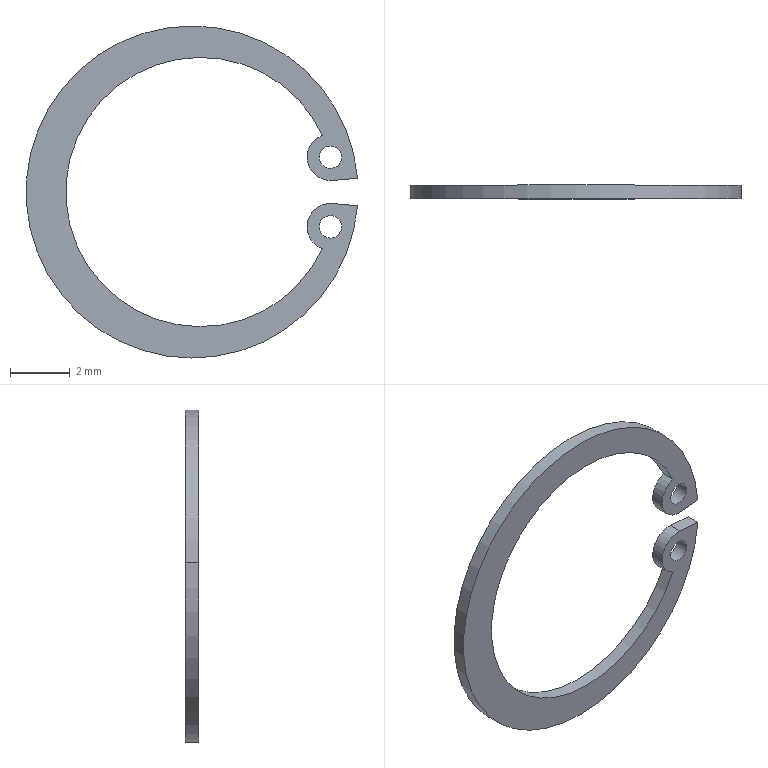Part | STEP file | 2026.6.15-Main Assembly图.sldasm-Part-286 | 1 solid | 16 faces | box 11.081 x 0.45 x 11.1 mm | volume 15.053 mm3 | cylinder 12 | plane 4 | commonest cylinder face diameters 0.75 x4 1.56 x4 9 x2 11.1 x2
STEP:
#1=CARTESIAN_POINT('',(-1507.657,1426.544,3408.546));
#2=VERTEX_POINT('',#1);
#3=CARTESIAN_POINT('',(-1508.494,1426.544,3408.473));
#4=VERTEX_POINT('',#3);
#5=CARTESIAN_POINT('',(-1508.494,1426.544,3408.473));
#6=DIRECTION('',(-0.9962,0.,-0.08716));
#7=VECTOR('',#6,1000.);
#8=LINE('',#5,#7);
#9=EDGE_CURVE('',#2,#4,#8,.T.);
#10=ORIENTED_EDGE('',*,*,#9,.T.);
#11=CARTESIAN_POINT('',(-1509.34,1426.544,3409.311));
#12=VERTEX_POINT('',#11);
#13=CARTESIAN_POINT('',(-1508.562,1426.544,3409.25));
#14=DIRECTION('',(0.,-1.,0.));
#15=DIRECTION('',(-0.9969,0.,0.0785));
#16=AXIS2_PLACEMENT_3D('',#13,#14,#15);
#17=CIRCLE('',#16,0.78);
#18=EDGE_CURVE('',#12,#4,#17,.T.);
#19=ORIENTED_EDGE('',*,*,#18,.F.);
#20=CARTESIAN_POINT('',(-1508.828,1426.544,3409.983));
#21=VERTEX_POINT('',#20);
#22=CARTESIAN_POINT('',(-1508.562,1426.544,3409.25));
#23=DIRECTION('',(0.,-1.,0.));
#24=DIRECTION('',(-0.9969,0.,0.0785));
#25=AXIS2_PLACEMENT_3D('',#22,#23,#24);
#26=CIRCLE('',#25,0.78);
#27=EDGE_CURVE('',#21,#12,#26,.T.);
#28=ORIENTED_EDGE('',*,*,#27,.F.);
#29=CARTESIAN_POINT('',(-1517.395,1426.544,3408.44));
#30=VERTEX_POINT('',#29);
#31=CARTESIAN_POINT('',(-1512.909,1426.544,3408.086));
#32=DIRECTION('',(0.,-1.,0.));
#33=DIRECTION('',(-0.9969,0.,0.0785));
#34=AXIS2_PLACEMENT_3D('',#31,#32,#33);
#35=CIRCLE('',#34,4.5);
#36=EDGE_CURVE('',#21,#30,#35,.T.);
#37=ORIENTED_EDGE('',*,*,#36,.T.);
#38=CARTESIAN_POINT('',(-1508.828,1426.544,3406.19));
#39=VERTEX_POINT('',#38);
#40=CARTESIAN_POINT('',(-1512.909,1426.544,3408.086));
#41=DIRECTION('',(0.,-1.,0.));
#42=DIRECTION('',(-0.9969,0.,0.0785));
#43=AXIS2_PLACEMENT_3D('',#40,#41,#42);
#44=CIRCLE('',#43,4.5);
#45=EDGE_CURVE('',#30,#39,#44,.T.);
#46=ORIENTED_EDGE('',*,*,#45,.T.);
#47=CARTESIAN_POINT('',(-1509.34,1426.544,3406.984));
#48=VERTEX_POINT('',#47);
#49=CARTESIAN_POINT('',(-1508.562,1426.544,3406.923));
#50=DIRECTION('',(0.,-1.,0.));
#51=DIRECTION('',(-0.9969,0.,0.0785));
#52=AXIS2_PLACEMENT_3D('',#49,#50,#51);
#53=CIRCLE('',#52,0.78);
#54=EDGE_CURVE('',#48,#39,#53,.T.);
#55=ORIENTED_EDGE('',*,*,#54,.F.);
#56=CARTESIAN_POINT('',(-1508.494,1426.544,3407.7));
#57=VERTEX_POINT('',#56);
#58=CARTESIAN_POINT('',(-1508.562,1426.544,3406.923));
#59=DIRECTION('',(0.,-1.,0.));
#60=DIRECTION('',(-0.9969,0.,0.0785));
#61=AXIS2_PLACEMENT_3D('',#58,#59,#60);
#62=CIRCLE('',#61,0.78);
#63=EDGE_CURVE('',#57,#48,#62,.T.);
#64=ORIENTED_EDGE('',*,*,#63,.F.);
#65=CARTESIAN_POINT('',(-1507.657,1426.544,3407.627));
#66=VERTEX_POINT('',#65);
#67=CARTESIAN_POINT('',(-1508.494,1426.544,3407.7));
#68=DIRECTION('',(0.9962,0.,-0.08716));
#69=VECTOR('',#68,1000.);
#70=LINE('',#67,#69);
#71=EDGE_CURVE('',#57,#66,#70,.T.);
#72=ORIENTED_EDGE('',*,*,#71,.T.);
#73=CARTESIAN_POINT('',(-1518.721,1426.544,3408.522));
#74=VERTEX_POINT('',#73);
#75=CARTESIAN_POINT('',(-1513.188,1426.544,3408.086));
#76=DIRECTION('',(0.,-1.,0.));
#77=DIRECTION('',(-0.9969,0.,0.0785));
#78=AXIS2_PLACEMENT_3D('',#75,#76,#77);
#79=CIRCLE('',#78,5.55);
#80=EDGE_CURVE('',#74,#66,#79,.T.);
#81=ORIENTED_EDGE('',*,*,#80,.F.);
#82=CARTESIAN_POINT('',(-1513.188,1426.544,3408.086));
#83=DIRECTION('',(0.,-1.,0.));
#84=DIRECTION('',(-0.9969,0.,0.0785));
#85=AXIS2_PLACEMENT_3D('',#82,#83,#84);
#86=CIRCLE('',#85,5.55);
#87=EDGE_CURVE('',#2,#74,#86,.T.);
#88=ORIENTED_EDGE('',*,*,#87,.F.);
#89=EDGE_LOOP('',(#10,#19,#28,#37,#46,#55,#64,#72,#81,#88));
#90=FACE_OUTER_BOUND('',#89,.T.);
#91=CARTESIAN_POINT('',(-1508.936,1426.544,3406.952));
#92=VERTEX_POINT('',#91);
#93=CARTESIAN_POINT('',(-1508.188,1426.544,3406.894));
#94=VERTEX_POINT('',#93);
#95=CARTESIAN_POINT('',(-1508.562,1426.544,3406.923));
#96=DIRECTION('',(0.,-1.,0.));
#97=DIRECTION('',(-0.9969,0.,0.0785));
#98=AXIS2_PLACEMENT_3D('',#95,#96,#97);
#99=CIRCLE('',#98,0.375);
#100=EDGE_CURVE('',#92,#94,#99,.T.);
#101=ORIENTED_EDGE('',*,*,#100,.T.);
#102=CARTESIAN_POINT('',(-1508.562,1426.544,3406.923));
#103=DIRECTION('',(0.,-1.,0.));
#104=DIRECTION('',(-0.9969,0.,0.0785));
#105=AXIS2_PLACEMENT_3D('',#102,#103,#104);
#106=CIRCLE('',#105,0.375);
#107=EDGE_CURVE('',#94,#92,#106,.T.);
#108=ORIENTED_EDGE('',*,*,#107,.T.);
#109=EDGE_LOOP('',(#101,#108));
#110=FACE_BOUND('',#109,.T.);
#111=CARTESIAN_POINT('',(-1508.936,1426.544,3409.279));
#112=VERTEX_POINT('',#111);
#113=CARTESIAN_POINT('',(-1508.188,1426.544,3409.22));
#114=VERTEX_POINT('',#113);
#115=CARTESIAN_POINT('',(-1508.562,1426.544,3409.25));
#116=DIRECTION('',(0.,-1.,0.));
#117=DIRECTION('',(-0.9969,0.,0.0785));
#118=AXIS2_PLACEMENT_3D('',#115,#116,#117);
#119=CIRCLE('',#118,0.375);
#120=EDGE_CURVE('',#112,#114,#119,.T.);
#121=ORIENTED_EDGE('',*,*,#120,.T.);
#122=CARTESIAN_POINT('',(-1508.562,1426.544,3409.25));
#123=DIRECTION('',(0.,-1.,0.));
#124=DIRECTION('',(-0.9969,0.,0.0785));
#125=AXIS2_PLACEMENT_3D('',#122,#123,#124);
#126=CIRCLE('',#125,0.375);
#127=EDGE_CURVE('',#114,#112,#126,.T.);
#128=ORIENTED_EDGE('',*,*,#127,.T.);
#129=EDGE_LOOP('',(#121,#128));
#130=FACE_BOUND('',#129,.T.);
#131=CARTESIAN_POINT('',(-1513.188,1426.544,3408.086));
#132=DIRECTION('',(0.,1.,0.));
#133=DIRECTION('',(0.,0.,-1.));
#134=AXIS2_PLACEMENT_3D('',#131,#132,#133);
#135=PLANE('',#134);
#136=ADVANCED_FACE('',(#90,#110,#130),#135,.T.);
#137=CARTESIAN_POINT('',(-1518.721,1426.094,3408.522));
#138=VERTEX_POINT('',#137);
#139=CARTESIAN_POINT('',(-1518.721,1426.094,3408.522));
#140=DIRECTION('',(0.,-1.,0.));
#141=VECTOR('',#140,1000.);
#142=LINE('',#139,#141);
#143=EDGE_CURVE('',#74,#138,#142,.T.);
#144=ORIENTED_EDGE('',*,*,#143,.F.);
#145=ORIENTED_EDGE('',*,*,#80,.T.);
#146=CARTESIAN_POINT('',(-1507.657,1426.094,3407.627));
#147=VERTEX_POINT('',#146);
#148=CARTESIAN_POINT('',(-1507.657,1406.528,3407.627));
#149=DIRECTION('',(0.,-1.,0.));
#150=VECTOR('',#149,1000.);
#151=LINE('',#148,#150);
#152=EDGE_CURVE('',#66,#147,#151,.T.);
#153=ORIENTED_EDGE('',*,*,#152,.T.);
#154=CARTESIAN_POINT('',(-1513.188,1426.094,3408.086));
#155=DIRECTION('',(0.,1.,0.));
#156=DIRECTION('',(-0.9969,0.,0.0785));
#157=AXIS2_PLACEMENT_3D('',#154,#155,#156);
#158=CIRCLE('',#157,5.55);
#159=EDGE_CURVE('',#147,#138,#158,.T.);
#160=ORIENTED_EDGE('',*,*,#159,.T.);
#161=EDGE_LOOP('',(#144,#145,#153,#160));
#162=FACE_OUTER_BOUND('',#161,.T.);
#163=CARTESIAN_POINT('',(-1513.188,1426.094,3408.086));
#164=DIRECTION('',(0.,-1.,0.));
#165=DIRECTION('',(0.9969,0.,-0.0785));
#166=AXIS2_PLACEMENT_3D('',#163,#164,#165);
#167=CYLINDRICAL_SURFACE('',#166,5.55);
#168=ADVANCED_FACE('',(#162),#167,.T.);
#169=CARTESIAN_POINT('',(-1508.494,1426.094,3408.473));
#170=VERTEX_POINT('',#169);
#171=CARTESIAN_POINT('',(-1508.494,1406.528,3408.473));
#172=DIRECTION('',(0.,-1.,0.));
#173=VECTOR('',#172,1000.);
#174=LINE('',#171,#173);
#175=EDGE_CURVE('',#4,#170,#174,.T.);
#176=ORIENTED_EDGE('',*,*,#175,.F.);
#177=ORIENTED_EDGE('',*,*,#9,.F.);
#178=CARTESIAN_POINT('',(-1507.657,1426.094,3408.546));
#179=VERTEX_POINT('',#178);
#180=CARTESIAN_POINT('',(-1507.657,1406.528,3408.546));
#181=DIRECTION('',(0.,1.,0.));
#182=VECTOR('',#181,1000.);
#183=LINE('',#180,#182);
#184=EDGE_CURVE('',#179,#2,#183,.T.);
#185=ORIENTED_EDGE('',*,*,#184,.F.);
#186=CARTESIAN_POINT('',(-1507.657,1426.094,3408.546));
#187=DIRECTION('',(-0.9962,0.,-0.08716));
#188=VECTOR('',#187,1000.);
#189=LINE('',#186,#188);
#190=EDGE_CURVE('',#179,#170,#189,.T.);
#191=ORIENTED_EDGE('',*,*,#190,.T.);
#192=EDGE_LOOP('',(#176,#177,#185,#191));
#193=FACE_OUTER_BOUND('',#192,.T.);
#194=CARTESIAN_POINT('',(-1508.494,1406.528,3408.473));
#195=DIRECTION('',(-0.08716,0.,0.9962));
#196=DIRECTION('',(0.,1.,0.));
#197=AXIS2_PLACEMENT_3D('',#194,#195,#196);
#198=PLANE('',#197);
#199=ADVANCED_FACE('',(#193),#198,.F.);
#200=CARTESIAN_POINT('',(-1509.34,1426.094,3409.311));
#201=VERTEX_POINT('',#200);
#202=CARTESIAN_POINT('',(-1509.34,1406.528,3409.311));
#203=DIRECTION('',(0.,-1.,0.));
#204=VECTOR('',#203,1000.);
#205=LINE('',#202,#204);
#206=EDGE_CURVE('',#12,#201,#205,.T.);
#207=ORIENTED_EDGE('',*,*,#206,.F.);
#208=ORIENTED_EDGE('',*,*,#18,.T.);
#209=ORIENTED_EDGE('',*,*,#175,.T.);
#210=CARTESIAN_POINT('',(-1508.562,1426.094,3409.25));
#211=DIRECTION('',(0.,1.,0.));
#212=DIRECTION('',(-0.9969,0.,0.0785));
#213=AXIS2_PLACEMENT_3D('',#210,#211,#212);
#214=CIRCLE('',#213,0.78);
#215=EDGE_CURVE('',#170,#201,#214,.T.);
#216=ORIENTED_EDGE('',*,*,#215,.T.);
#217=EDGE_LOOP('',(#207,#208,#209,#216));
#218=FACE_OUTER_BOUND('',#217,.T.);
#219=CARTESIAN_POINT('',(-1508.562,1406.528,3409.25));
#220=DIRECTION('',(0.,-1.,0.));
#221=DIRECTION('',(0.9969,0.,-0.0785));
#222=AXIS2_PLACEMENT_3D('',#219,#220,#221);
#223=CYLINDRICAL_SURFACE('',#222,0.78);
#224=ADVANCED_FACE('',(#218),#223,.T.);
#225=CARTESIAN_POINT('',(-1517.395,1426.094,3408.44));
#226=VERTEX_POINT('',#225);
#227=CARTESIAN_POINT('',(-1517.395,1406.528,3408.44));
#228=DIRECTION('',(0.,-1.,0.));
#229=VECTOR('',#228,1000.);
#230=LINE('',#227,#229);
#231=EDGE_CURVE('',#30,#226,#230,.T.);
#232=ORIENTED_EDGE('',*,*,#231,.F.);
#233=ORIENTED_EDGE('',*,*,#36,.F.);
#234=CARTESIAN_POINT('',(-1508.828,1426.094,3409.983));
#235=VERTEX_POINT('',#234);
#236=CARTESIAN_POINT('',(-1508.828,1406.528,3409.983));
#237=DIRECTION('',(0.,1.,0.));
#238=VECTOR('',#237,1000.);
#239=LINE('',#236,#238);
#240=EDGE_CURVE('',#235,#21,#239,.T.);
#241=ORIENTED_EDGE('',*,*,#240,.F.);
#242=CARTESIAN_POINT('',(-1512.909,1426.094,3408.086));
#243=DIRECTION('',(0.,-1.,0.));
#244=DIRECTION('',(-0.9969,0.,0.0785));
#245=AXIS2_PLACEMENT_3D('',#242,#243,#244);
#246=CIRCLE('',#245,4.5);
#247=EDGE_CURVE('',#235,#226,#246,.T.);
#248=ORIENTED_EDGE('',*,*,#247,.T.);
#249=EDGE_LOOP('',(#232,#233,#241,#248));
#250=FACE_OUTER_BOUND('',#249,.T.);
#251=CARTESIAN_POINT('',(-1512.909,1406.528,3408.086));
#252=DIRECTION('',(0.,-1.,0.));
#253=DIRECTION('',(0.9969,0.,-0.0785));
#254=AXIS2_PLACEMENT_3D('',#251,#252,#253);
#255=CYLINDRICAL_SURFACE('',#254,4.5);
#256=ADVANCED_FACE('',(#250),#255,.F.);
#257=CARTESIAN_POINT('',(-1509.34,1426.094,3406.984));
#258=VERTEX_POINT('',#257);
#259=CARTESIAN_POINT('',(-1509.34,1406.528,3406.984));
#260=DIRECTION('',(0.,-1.,0.));
#261=VECTOR('',#260,1000.);
#262=LINE('',#259,#261);
#263=EDGE_CURVE('',#48,#258,#262,.T.);
#264=ORIENTED_EDGE('',*,*,#263,.F.);
#265=ORIENTED_EDGE('',*,*,#54,.T.);
#266=CARTESIAN_POINT('',(-1508.828,1426.094,3406.19));
#267=VERTEX_POINT('',#266);
#268=CARTESIAN_POINT('',(-1508.828,1406.528,3406.19));
#269=DIRECTION('',(0.,-1.,0.));
#270=VECTOR('',#269,1000.);
#271=LINE('',#268,#270);
#272=EDGE_CURVE('',#39,#267,#271,.T.);
#273=ORIENTED_EDGE('',*,*,#272,.T.);
#274=CARTESIAN_POINT('',(-1508.562,1426.094,3406.923));
#275=DIRECTION('',(0.,1.,0.));
#276=DIRECTION('',(-0.9969,0.,0.0785));
#277=AXIS2_PLACEMENT_3D('',#274,#275,#276);
#278=CIRCLE('',#277,0.78);
#279=EDGE_CURVE('',#267,#258,#278,.T.);
#280=ORIENTED_EDGE('',*,*,#279,.T.);
#281=EDGE_LOOP('',(#264,#265,#273,#280));
#282=FACE_OUTER_BOUND('',#281,.T.);
#283=CARTESIAN_POINT('',(-1508.562,1406.528,3406.923));
#284=DIRECTION('',(0.,-1.,0.));
#285=DIRECTION('',(0.9969,0.,-0.0785));
#286=AXIS2_PLACEMENT_3D('',#283,#284,#285);
#287=CYLINDRICAL_SURFACE('',#286,0.78);
#288=ADVANCED_FACE('',(#282),#287,.T.);
#289=CARTESIAN_POINT('',(-1508.494,1426.094,3407.7));
#290=VERTEX_POINT('',#289);
#291=CARTESIAN_POINT('',(-1508.494,1406.528,3407.7));
#292=DIRECTION('',(0.,1.,0.));
#293=VECTOR('',#292,1000.);
#294=LINE('',#291,#293);
#295=EDGE_CURVE('',#290,#57,#294,.T.);
#296=ORIENTED_EDGE('',*,*,#295,.F.);
#297=CARTESIAN_POINT('',(-1508.494,1426.094,3407.7));
#298=DIRECTION('',(0.9962,0.,-0.08716));
#299=VECTOR('',#298,1000.);
#300=LINE('',#297,#299);
#301=EDGE_CURVE('',#290,#147,#300,.T.);
#302=ORIENTED_EDGE('',*,*,#301,.T.);
#303=ORIENTED_EDGE('',*,*,#152,.F.);
#304=ORIENTED_EDGE('',*,*,#71,.F.);
#305=EDGE_LOOP('',(#296,#302,#303,#304));
#306=FACE_OUTER_BOUND('',#305,.T.);
#307=CARTESIAN_POINT('',(-1508.494,1406.528,3407.7));
#308=DIRECTION('',(-0.08716,0.,-0.9962));
#309=DIRECTION('',(0.,1.,0.));
#310=AXIS2_PLACEMENT_3D('',#307,#308,#309);
#311=PLANE('',#310);
#312=ADVANCED_FACE('',(#306),#311,.F.);
#313=CARTESIAN_POINT('',(-1508.188,1426.094,3406.894));
#314=VERTEX_POINT('',#313);
#315=CARTESIAN_POINT('',(-1508.188,1410.854,3406.894));
#316=DIRECTION('',(0.,1.,0.));
#317=VECTOR('',#316,1000.);
#318=LINE('',#315,#317);
#319=EDGE_CURVE('',#314,#94,#318,.T.);
#320=ORIENTED_EDGE('',*,*,#319,.T.);
#321=ORIENTED_EDGE('',*,*,#100,.F.);
#322=CARTESIAN_POINT('',(-1508.936,1426.094,3406.952));
#323=VERTEX_POINT('',#322);
#324=CARTESIAN_POINT('',(-1508.936,1410.854,3406.952));
#325=DIRECTION('',(0.,1.,0.));
#326=VECTOR('',#325,1000.);
#327=LINE('',#324,#326);
#328=EDGE_CURVE('',#323,#92,#327,.T.);
#329=ORIENTED_EDGE('',*,*,#328,.F.);
#330=CARTESIAN_POINT('',(-1508.562,1426.094,3406.923));
#331=DIRECTION('',(0.,-1.,0.));
#332=DIRECTION('',(-0.9969,0.,0.0785));
#333=AXIS2_PLACEMENT_3D('',#330,#331,#332);
#334=CIRCLE('',#333,0.375);
#335=EDGE_CURVE('',#323,#314,#334,.T.);
#336=ORIENTED_EDGE('',*,*,#335,.T.);
#337=EDGE_LOOP('',(#320,#321,#329,#336));
#338=FACE_OUTER_BOUND('',#337,.T.);
#339=CARTESIAN_POINT('',(-1508.562,1410.854,3406.923));
#340=DIRECTION('',(0.,-1.,0.));
#341=DIRECTION('',(0.9969,0.,-0.0785));
#342=AXIS2_PLACEMENT_3D('',#339,#340,#341);
#343=CYLINDRICAL_SURFACE('',#342,0.375);
#344=ADVANCED_FACE('',(#338),#343,.F.);
#345=CARTESIAN_POINT('',(-1508.188,1426.094,3409.22));
#346=VERTEX_POINT('',#345);
#347=CARTESIAN_POINT('',(-1508.188,1410.854,3409.22));
#348=DIRECTION('',(0.,1.,0.));
#349=VECTOR('',#348,1000.);
#350=LINE('',#347,#349);
#351=EDGE_CURVE('',#346,#114,#350,.T.);
#352=ORIENTED_EDGE('',*,*,#351,.T.);
#353=ORIENTED_EDGE('',*,*,#120,.F.);
#354=CARTESIAN_POINT('',(-1508.936,1426.094,3409.279));
#355=VERTEX_POINT('',#354);
#356=CARTESIAN_POINT('',(-1508.936,1410.854,3409.279));
#357=DIRECTION('',(0.,1.,0.));
#358=VECTOR('',#357,1000.);
#359=LINE('',#356,#358);
#360=EDGE_CURVE('',#355,#112,#359,.T.);
#361=ORIENTED_EDGE('',*,*,#360,.F.);
#362=CARTESIAN_POINT('',(-1508.562,1426.094,3409.25));
#363=DIRECTION('',(0.,-1.,0.));
#364=DIRECTION('',(-0.9969,0.,0.0785));
#365=AXIS2_PLACEMENT_3D('',#362,#363,#364);
#366=CIRCLE('',#365,0.375);
#367=EDGE_CURVE('',#355,#346,#366,.T.);
#368=ORIENTED_EDGE('',*,*,#367,.T.);
#369=EDGE_LOOP('',(#352,#353,#361,#368));
#370=FACE_OUTER_BOUND('',#369,.T.);
#371=CARTESIAN_POINT('',(-1508.562,1410.854,3409.25));
#372=DIRECTION('',(0.,-1.,0.));
#373=DIRECTION('',(0.9969,0.,-0.0785));
#374=AXIS2_PLACEMENT_3D('',#371,#372,#373);
#375=CYLINDRICAL_SURFACE('',#374,0.375);
#376=ADVANCED_FACE('',(#370),#375,.F.);
#377=ORIENTED_EDGE('',*,*,#301,.F.);
#378=CARTESIAN_POINT('',(-1508.562,1426.094,3406.923));
#379=DIRECTION('',(0.,1.,0.));
#380=DIRECTION('',(-0.9969,0.,0.0785));
#381=AXIS2_PLACEMENT_3D('',#378,#379,#380);
#382=CIRCLE('',#381,0.78);
#383=EDGE_CURVE('',#258,#290,#382,.T.);
#384=ORIENTED_EDGE('',*,*,#383,.F.);
#385=ORIENTED_EDGE('',*,*,#279,.F.);
#386=CARTESIAN_POINT('',(-1512.909,1426.094,3408.086));
#387=DIRECTION('',(0.,-1.,0.));
#388=DIRECTION('',(-0.9969,0.,0.0785));
#389=AXIS2_PLACEMENT_3D('',#386,#387,#388);
#390=CIRCLE('',#389,4.5);
#391=EDGE_CURVE('',#226,#267,#390,.T.);
#392=ORIENTED_EDGE('',*,*,#391,.F.);
#393=ORIENTED_EDGE('',*,*,#247,.F.);
#394=CARTESIAN_POINT('',(-1508.562,1426.094,3409.25));
#395=DIRECTION('',(0.,1.,0.));
#396=DIRECTION('',(-0.9969,0.,0.0785));
#397=AXIS2_PLACEMENT_3D('',#394,#395,#396);
#398=CIRCLE('',#397,0.78);
#399=EDGE_CURVE('',#201,#235,#398,.T.);
#400=ORIENTED_EDGE('',*,*,#399,.F.);
#401=ORIENTED_EDGE('',*,*,#215,.F.);
#402=ORIENTED_EDGE('',*,*,#190,.F.);
#403=CARTESIAN_POINT('',(-1513.188,1426.094,3408.086));
#404=DIRECTION('',(0.,1.,0.));
#405=DIRECTION('',(-0.9969,0.,0.0785));
#406=AXIS2_PLACEMENT_3D('',#403,#404,#405);
#407=CIRCLE('',#406,5.55);
#408=EDGE_CURVE('',#138,#179,#407,.T.);
#409=ORIENTED_EDGE('',*,*,#408,.F.);
#410=ORIENTED_EDGE('',*,*,#159,.F.);
#411=EDGE_LOOP('',(#377,#384,#385,#392,#393,#400,#401,#402,#409,#410));
#412=FACE_OUTER_BOUND('',#411,.T.);
#413=ORIENTED_EDGE('',*,*,#335,.F.);
#414=CARTESIAN_POINT('',(-1508.562,1426.094,3406.923));
#415=DIRECTION('',(0.,-1.,0.));
#416=DIRECTION('',(-0.9969,0.,0.0785));
#417=AXIS2_PLACEMENT_3D('',#414,#415,#416);
#418=CIRCLE('',#417,0.375);
#419=EDGE_CURVE('',#314,#323,#418,.T.);
#420=ORIENTED_EDGE('',*,*,#419,.F.);
#421=EDGE_LOOP('',(#413,#420));
#422=FACE_BOUND('',#421,.T.);
#423=ORIENTED_EDGE('',*,*,#367,.F.);
#424=CARTESIAN_POINT('',(-1508.562,1426.094,3409.25));
#425=DIRECTION('',(0.,-1.,0.));
#426=DIRECTION('',(-0.9969,0.,0.0785));
#427=AXIS2_PLACEMENT_3D('',#424,#425,#426);
#428=CIRCLE('',#427,0.375);
#429=EDGE_CURVE('',#346,#355,#428,.T.);
#430=ORIENTED_EDGE('',*,*,#429,.F.);
#431=EDGE_LOOP('',(#423,#430));
#432=FACE_BOUND('',#431,.T.);
#433=CARTESIAN_POINT('',(-1513.188,1426.094,3408.086));
#434=DIRECTION('',(0.,1.,0.));
#435=DIRECTION('',(0.,0.,-1.));
#436=AXIS2_PLACEMENT_3D('',#433,#434,#435);
#437=PLANE('',#436);
#438=ADVANCED_FACE('',(#412,#422,#432),#437,.F.);
#439=ORIENTED_EDGE('',*,*,#87,.T.);
#440=ORIENTED_EDGE('',*,*,#143,.T.);
#441=ORIENTED_EDGE('',*,*,#408,.T.);
#442=ORIENTED_EDGE('',*,*,#184,.T.);
#443=EDGE_LOOP('',(#439,#440,#441,#442));
#444=FACE_OUTER_BOUND('',#443,.T.);
#445=CARTESIAN_POINT('',(-1513.188,1426.094,3408.086));
#446=DIRECTION('',(0.,-1.,0.));
#447=DIRECTION('',(0.9969,0.,-0.0785));
#448=AXIS2_PLACEMENT_3D('',#445,#446,#447);
#449=CYLINDRICAL_SURFACE('',#448,5.55);
#450=ADVANCED_FACE('',(#444),#449,.T.);
#451=ORIENTED_EDGE('',*,*,#27,.T.);
#452=ORIENTED_EDGE('',*,*,#206,.T.);
#453=ORIENTED_EDGE('',*,*,#399,.T.);
#454=ORIENTED_EDGE('',*,*,#240,.T.);
#455=EDGE_LOOP('',(#451,#452,#453,#454));
#456=FACE_OUTER_BOUND('',#455,.T.);
#457=CARTESIAN_POINT('',(-1508.562,1406.528,3409.25));
#458=DIRECTION('',(0.,-1.,0.));
#459=DIRECTION('',(0.9969,0.,-0.0785));
#460=AXIS2_PLACEMENT_3D('',#457,#458,#459);
#461=CYLINDRICAL_SURFACE('',#460,0.78);
#462=ADVANCED_FACE('',(#456),#461,.T.);
#463=ORIENTED_EDGE('',*,*,#45,.F.);
#464=ORIENTED_EDGE('',*,*,#231,.T.);
#465=ORIENTED_EDGE('',*,*,#391,.T.);
#466=ORIENTED_EDGE('',*,*,#272,.F.);
#467=EDGE_LOOP('',(#463,#464,#465,#466));
#468=FACE_OUTER_BOUND('',#467,.T.);
#469=CARTESIAN_POINT('',(-1512.909,1406.528,3408.086));
#470=DIRECTION('',(0.,-1.,0.));
#471=DIRECTION('',(0.9969,0.,-0.0785));
#472=AXIS2_PLACEMENT_3D('',#469,#470,#471);
#473=CYLINDRICAL_SURFACE('',#472,4.5);
#474=ADVANCED_FACE('',(#468),#473,.F.);
#475=ORIENTED_EDGE('',*,*,#63,.T.);
#476=ORIENTED_EDGE('',*,*,#263,.T.);
#477=ORIENTED_EDGE('',*,*,#383,.T.);
#478=ORIENTED_EDGE('',*,*,#295,.T.);
#479=EDGE_LOOP('',(#475,#476,#477,#478));
#480=FACE_OUTER_BOUND('',#479,.T.);
#481=CARTESIAN_POINT('',(-1508.562,1406.528,3406.923));
#482=DIRECTION('',(0.,-1.,0.));
#483=DIRECTION('',(0.9969,0.,-0.0785));
#484=AXIS2_PLACEMENT_3D('',#481,#482,#483);
#485=CYLINDRICAL_SURFACE('',#484,0.78);
#486=ADVANCED_FACE('',(#480),#485,.T.);
#487=ORIENTED_EDGE('',*,*,#107,.F.);
#488=ORIENTED_EDGE('',*,*,#319,.F.);
#489=ORIENTED_EDGE('',*,*,#419,.T.);
#490=ORIENTED_EDGE('',*,*,#328,.T.);
#491=EDGE_LOOP('',(#487,#488,#489,#490));
#492=FACE_OUTER_BOUND('',#491,.T.);
#493=CARTESIAN_POINT('',(-1508.562,1410.854,3406.923));
#494=DIRECTION('',(0.,-1.,0.));
#495=DIRECTION('',(0.9969,0.,-0.0785));
#496=AXIS2_PLACEMENT_3D('',#493,#494,#495);
#497=CYLINDRICAL_SURFACE('',#496,0.375);
#498=ADVANCED_FACE('',(#492),#497,.F.);
#499=ORIENTED_EDGE('',*,*,#127,.F.);
#500=ORIENTED_EDGE('',*,*,#351,.F.);
#501=ORIENTED_EDGE('',*,*,#429,.T.);
#502=ORIENTED_EDGE('',*,*,#360,.T.);
#503=EDGE_LOOP('',(#499,#500,#501,#502));
#504=FACE_OUTER_BOUND('',#503,.T.);
#505=CARTESIAN_POINT('',(-1508.562,1410.854,3409.25));
#506=DIRECTION('',(0.,-1.,0.));
#507=DIRECTION('',(0.9969,0.,-0.0785));
#508=AXIS2_PLACEMENT_3D('',#505,#506,#507);
#509=CYLINDRICAL_SURFACE('',#508,0.375);
#510=ADVANCED_FACE('',(#504),#509,.F.);
#511=CLOSED_SHELL('',(#136,#168,#199,#224,#256,#288,#312,#344,#376,#438,#450,#462,#474,#486,#498,#510));
#512=MANIFOLD_SOLID_BREP('',#511);
#513=CARTESIAN_POINT('',(0.,0.,0.));
#514=DIRECTION('',(0.,0.,1.));
#515=DIRECTION('',(1.,0.,0.));
#516=AXIS2_PLACEMENT_3D('',#513,#514,#515);
#517=(LENGTH_UNIT()NAMED_UNIT(*)SI_UNIT(.MILLI.,.METRE.));
#518=UNCERTAINTY_MEASURE_WITH_UNIT(LENGTH_MEASURE(0.00001),#517,'','');
#519=(NAMED_UNIT(*)PLANE_ANGLE_UNIT()SI_UNIT($,.RADIAN.));
#520=(NAMED_UNIT(*)SI_UNIT($,.STERADIAN.)SOLID_ANGLE_UNIT());
#521=(GEOMETRIC_REPRESENTATION_CONTEXT(3)GLOBAL_UNCERTAINTY_ASSIGNED_CONTEXT((#518))GLOBAL_UNIT_ASSIGNED_CONTEXT((#517,#519,#520))REPRESENTATION_CONTEXT('',''));
#522=ADVANCED_BREP_SHAPE_REPRESENTATION('',(#512,#516),#521);